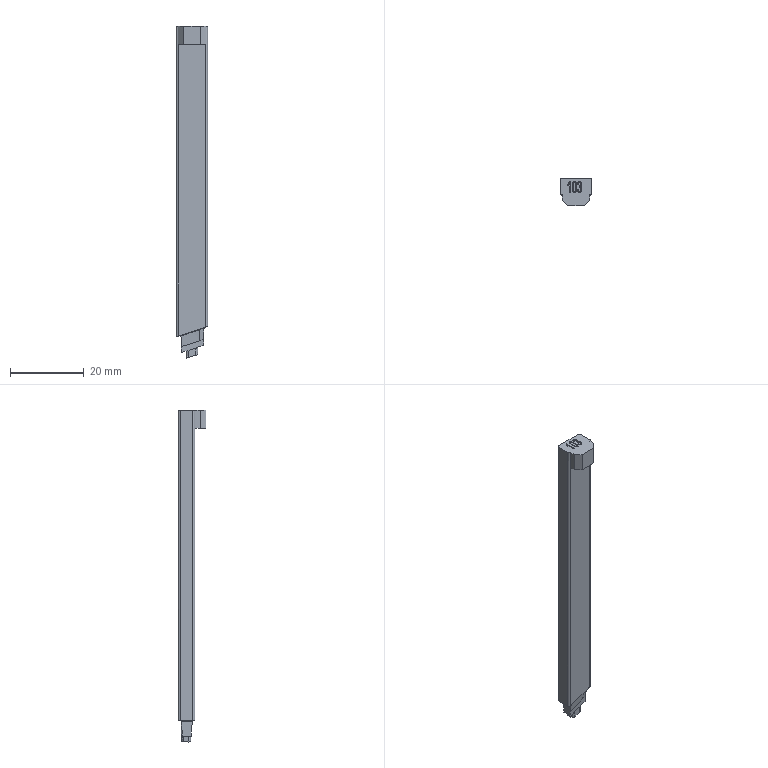Part | Creo | 1 solid | 77 faces | box 8.5 x 7.5 x 90.23 mm | volume 3355 mm3 | plane 31 | cylinder 16 | other 16 | spline 13 | cone 1 | commonest cylinder face diameters 1 x5 1.005 x2 114.945 x2 116.698 x1 118.069 x1 118.661 x1